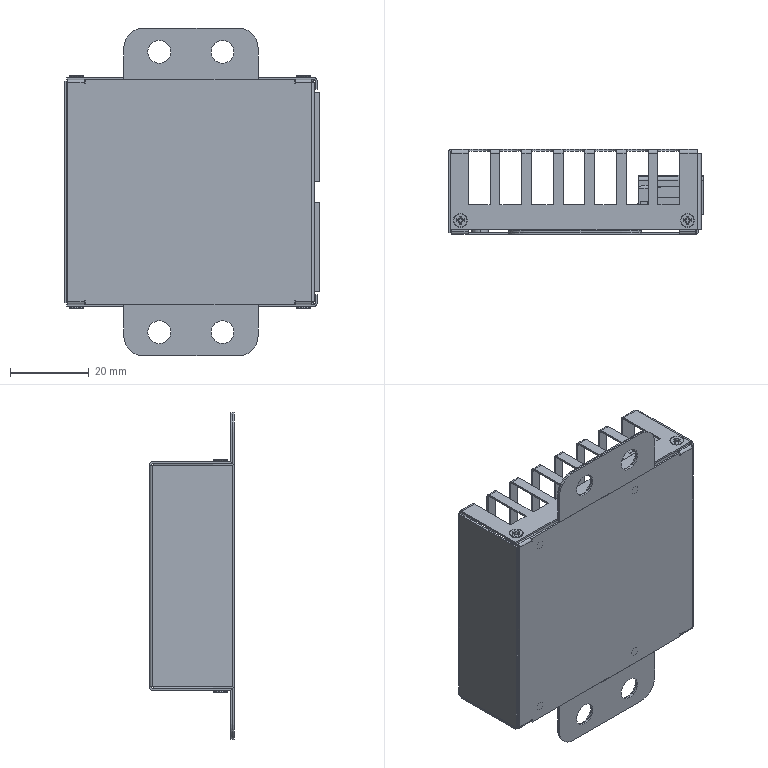Part | NX | features BREP 6 | 9 solids | 2852 faces | box 64.47 x 21.5 x 83 mm | volume 11085 mm3 | plane 1326 | cylinder 818 | spline 628 | cone 48 | torus 32 | commonest cylinder face diameters 2.013 x168 0.4 x124 1.567 x116 2.5 x64 1.6 x40 2 x40